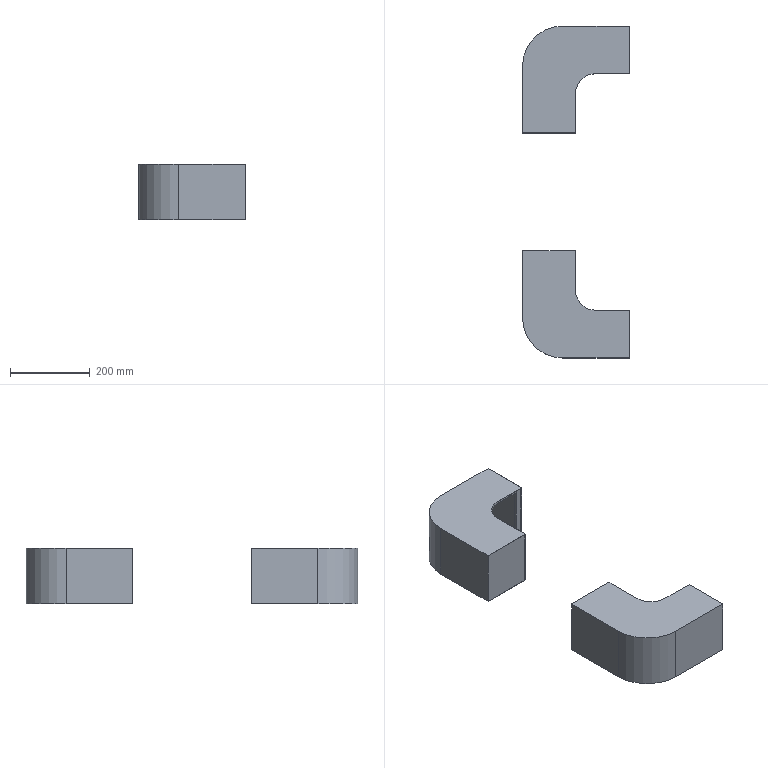Part | NX | features BREP 3 | 3 solids | 72 faces | box 267.373 x 830 x 140 mm | volume 2977877 mm3 | plane 54 | cylinder 18 | commonest cylinder face diameters 10 x6 100 x6 190 x3 200 x3